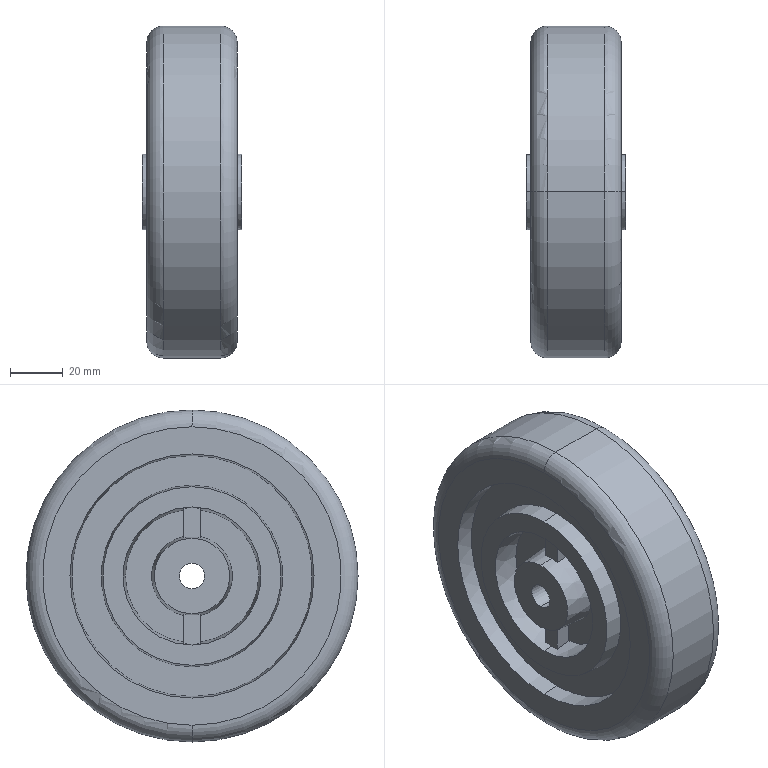Part | SolidWorks | features Cut 2, Draft 2, ICE 2, BossThin 1, Extrusion 1, Fillet 1, MirrorPattern 1 | 1 solid | 41 faces | box 37.592 x 125.73 x 125.73 mm | volume 351247 mm3 | plane 17 | cone 16 | cylinder 4 | torus 4 | commonest cylinder face diameters 9.652 x2 125.73 x2
STEP:
#1=CARTESIAN_POINT('',(18.796,-76.2,-39.751));
#2=VERTEX_POINT('',#1);
#3=CARTESIAN_POINT('',(18.796,-76.2,-30.099));
#4=VERTEX_POINT('',#3);
#5=CARTESIAN_POINT('',(18.796,-76.2,-34.925));
#6=DIRECTION('',(-1.,0.,0.));
#7=DIRECTION('',(0.,0.,1.));
#8=AXIS2_PLACEMENT_3D('',#5,#6,#7);
#9=CIRCLE('',#8,4.826);
#10=EDGE_CURVE('',#2,#4,#9,.T.);
#11=ORIENTED_EDGE('',*,*,#10,.F.);
#12=CARTESIAN_POINT('',(-18.796,-76.2,-39.751));
#13=VERTEX_POINT('',#12);
#14=CARTESIAN_POINT('',(18.796,-76.2,-39.751));
#15=DIRECTION('',(-1.,0.,0.));
#16=VECTOR('',#15,1000.);
#17=LINE('',#14,#16);
#18=EDGE_CURVE('',#2,#13,#17,.T.);
#19=ORIENTED_EDGE('',*,*,#18,.T.);
#20=CARTESIAN_POINT('',(-18.796,-76.2,-30.099));
#21=VERTEX_POINT('',#20);
#22=CARTESIAN_POINT('',(-18.796,-76.2,-34.925));
#23=DIRECTION('',(-1.,0.,0.));
#24=DIRECTION('',(0.,0.,1.));
#25=AXIS2_PLACEMENT_3D('',#22,#23,#24);
#26=CIRCLE('',#25,4.826);
#27=EDGE_CURVE('',#13,#21,#26,.T.);
#28=ORIENTED_EDGE('',*,*,#27,.T.);
#29=CARTESIAN_POINT('',(18.796,-76.2,-30.099));
#30=DIRECTION('',(-1.,0.,0.));
#31=VECTOR('',#30,1000.);
#32=LINE('',#29,#31);
#33=EDGE_CURVE('',#4,#21,#32,.T.);
#34=ORIENTED_EDGE('',*,*,#33,.F.);
#35=EDGE_LOOP('',(#11,#19,#28,#34));
#36=FACE_OUTER_BOUND('',#35,.T.);
#37=CARTESIAN_POINT('',(18.796,-76.2,-34.925));
#38=DIRECTION('',(-1.,0.,0.));
#39=DIRECTION('',(0.,0.,1.));
#40=AXIS2_PLACEMENT_3D('',#37,#38,#39);
#41=CYLINDRICAL_SURFACE('',#40,4.826);
#42=ADVANCED_FACE('',(#36),#41,.F.);
#43=CARTESIAN_POINT('',(10.795,-76.2,27.94));
#44=VERTEX_POINT('',#43);
#45=CARTESIAN_POINT('',(10.795,-76.2,-97.79));
#46=VERTEX_POINT('',#45);
#47=CARTESIAN_POINT('',(10.795,-76.2,-34.925));
#48=DIRECTION('',(-1.,0.,0.));
#49=DIRECTION('',(0.,0.,-1.));
#50=AXIS2_PLACEMENT_3D('',#47,#48,#49);
#51=CIRCLE('',#50,62.865);
#52=EDGE_CURVE('',#44,#46,#51,.T.);
#53=ORIENTED_EDGE('',*,*,#52,.F.);
#54=CARTESIAN_POINT('',(17.145,-76.2,21.59));
#55=VERTEX_POINT('',#54);
#56=CARTESIAN_POINT('',(10.795,-76.2,21.59));
#57=DIRECTION('',(0.,1.,0.));
#58=DIRECTION('',(0.,0.,1.));
#59=AXIS2_PLACEMENT_3D('',#56,#57,#58);
#60=CIRCLE('',#59,6.35);
#61=EDGE_CURVE('',#44,#55,#60,.T.);
#62=ORIENTED_EDGE('',*,*,#61,.T.);
#63=CARTESIAN_POINT('',(17.145,-76.2,-91.44));
#64=VERTEX_POINT('',#63);
#65=CARTESIAN_POINT('',(17.145,-76.2,-34.925));
#66=DIRECTION('',(1.,0.,0.));
#67=DIRECTION('',(0.,0.,-1.));
#68=AXIS2_PLACEMENT_3D('',#65,#66,#67);
#69=CIRCLE('',#68,56.515);
#70=EDGE_CURVE('',#64,#55,#69,.T.);
#71=ORIENTED_EDGE('',*,*,#70,.F.);
#72=CARTESIAN_POINT('',(10.795,-76.2,-91.44));
#73=DIRECTION('',(0.,-1.,0.));
#74=DIRECTION('',(0.,0.,-1.));
#75=AXIS2_PLACEMENT_3D('',#72,#73,#74);
#76=CIRCLE('',#75,6.35);
#77=EDGE_CURVE('',#46,#64,#76,.T.);
#78=ORIENTED_EDGE('',*,*,#77,.F.);
#79=EDGE_LOOP('',(#53,#62,#71,#78));
#80=FACE_OUTER_BOUND('',#79,.T.);
#81=CARTESIAN_POINT('',(10.795,-76.2,-34.925));
#82=DIRECTION('',(1.,0.,0.));
#83=DIRECTION('',(0.,0.,-1.));
#84=AXIS2_PLACEMENT_3D('',#81,#82,#83);
#85=TOROIDAL_SURFACE('',#84,56.515,6.35);
#86=ADVANCED_FACE('',(#80),#85,.T.);
#87=CARTESIAN_POINT('',(-17.145,-76.2,21.59));
#88=VERTEX_POINT('',#87);
#89=CARTESIAN_POINT('',(-17.145,-76.2,-91.44));
#90=VERTEX_POINT('',#89);
#91=CARTESIAN_POINT('',(-17.145,-76.2,-34.925));
#92=DIRECTION('',(-1.,0.,0.));
#93=DIRECTION('',(0.,0.,-1.));
#94=AXIS2_PLACEMENT_3D('',#91,#92,#93);
#95=CIRCLE('',#94,56.515);
#96=EDGE_CURVE('',#88,#90,#95,.T.);
#97=ORIENTED_EDGE('',*,*,#96,.F.);
#98=CARTESIAN_POINT('',(-10.795,-76.2,27.94));
#99=VERTEX_POINT('',#98);
#100=CARTESIAN_POINT('',(-10.795,-76.2,21.59));
#101=DIRECTION('',(0.,1.,0.));
#102=DIRECTION('',(0.,0.,1.));
#103=AXIS2_PLACEMENT_3D('',#100,#101,#102);
#104=CIRCLE('',#103,6.35);
#105=EDGE_CURVE('',#88,#99,#104,.T.);
#106=ORIENTED_EDGE('',*,*,#105,.T.);
#107=CARTESIAN_POINT('',(-10.795,-76.2,-97.79));
#108=VERTEX_POINT('',#107);
#109=CARTESIAN_POINT('',(-10.795,-76.2,-34.925));
#110=DIRECTION('',(1.,0.,0.));
#111=DIRECTION('',(0.,0.,-1.));
#112=AXIS2_PLACEMENT_3D('',#109,#110,#111);
#113=CIRCLE('',#112,62.865);
#114=EDGE_CURVE('',#108,#99,#113,.T.);
#115=ORIENTED_EDGE('',*,*,#114,.F.);
#116=CARTESIAN_POINT('',(-10.795,-76.2,-91.44));
#117=DIRECTION('',(0.,-1.,0.));
#118=DIRECTION('',(0.,0.,-1.));
#119=AXIS2_PLACEMENT_3D('',#116,#117,#118);
#120=CIRCLE('',#119,6.35);
#121=EDGE_CURVE('',#90,#108,#120,.T.);
#122=ORIENTED_EDGE('',*,*,#121,.F.);
#123=EDGE_LOOP('',(#97,#106,#115,#122));
#124=FACE_OUTER_BOUND('',#123,.T.);
#125=CARTESIAN_POINT('',(-10.795,-76.2,-34.925));
#126=DIRECTION('',(1.,0.,0.));
#127=DIRECTION('',(0.,0.,-1.));
#128=AXIS2_PLACEMENT_3D('',#125,#126,#127);
#129=TOROIDAL_SURFACE('',#128,56.515,6.35);
#130=ADVANCED_FACE('',(#124),#129,.T.);
#131=CARTESIAN_POINT('',(18.796,-76.2,-20.637));
#132=VERTEX_POINT('',#131);
#133=CARTESIAN_POINT('',(18.796,-76.2,-49.213));
#134=VERTEX_POINT('',#133);
#135=CARTESIAN_POINT('',(18.796,-76.2,-34.925));
#136=DIRECTION('',(1.,0.,0.));
#137=DIRECTION('',(0.,0.,-1.));
#138=AXIS2_PLACEMENT_3D('',#135,#136,#137);
#139=CIRCLE('',#138,14.288);
#140=EDGE_CURVE('',#132,#134,#139,.T.);
#141=ORIENTED_EDGE('',*,*,#140,.F.);
#142=CARTESIAN_POINT('',(6.985,-76.2,-19.604));
#143=VERTEX_POINT('',#142);
#144=CARTESIAN_POINT('',(18.796,-76.2,-20.638));
#145=DIRECTION('',(-0.9962,0.,0.08716));
#146=VECTOR('',#145,1000.);
#147=LINE('',#144,#146);
#148=EDGE_CURVE('',#132,#143,#147,.T.);
#149=ORIENTED_EDGE('',*,*,#148,.T.);
#150=CARTESIAN_POINT('',(6.985,-76.2,-50.246));
#151=VERTEX_POINT('',#150);
#152=CARTESIAN_POINT('',(6.985,-76.2,-34.925));
#153=DIRECTION('',(1.,0.,0.));
#154=DIRECTION('',(0.,0.,-1.));
#155=AXIS2_PLACEMENT_3D('',#152,#153,#154);
#156=CIRCLE('',#155,15.321);
#157=EDGE_CURVE('',#143,#151,#156,.T.);
#158=ORIENTED_EDGE('',*,*,#157,.T.);
#159=CARTESIAN_POINT('',(18.796,-76.2,-49.213));
#160=DIRECTION('',(-0.9962,0.,-0.08716));
#161=VECTOR('',#160,1000.);
#162=LINE('',#159,#161);
#163=EDGE_CURVE('',#134,#151,#162,.T.);
#164=ORIENTED_EDGE('',*,*,#163,.F.);
#165=EDGE_LOOP('',(#141,#149,#158,#164));
#166=FACE_OUTER_BOUND('',#165,.T.);
#167=CARTESIAN_POINT('',(18.796,-76.2,-34.925));
#168=DIRECTION('',(-1.,0.,0.));
#169=DIRECTION('',(0.,0.,-1.));
#170=AXIS2_PLACEMENT_3D('',#167,#168,#169);
#171=CONICAL_SURFACE('',#170,14.288,0.08727);
#172=ADVANCED_FACE('',(#166),#171,.T.);
#173=CARTESIAN_POINT('',(6.985,-76.2,-60.181));
#174=VERTEX_POINT('',#173);
#175=CARTESIAN_POINT('',(6.985,-76.2,-9.669));
#176=VERTEX_POINT('',#175);
#177=CARTESIAN_POINT('',(6.985,-76.2,-34.925));
#178=DIRECTION('',(-1.,0.,0.));
#179=DIRECTION('',(0.,0.,-1.));
#180=AXIS2_PLACEMENT_3D('',#177,#178,#179);
#181=CIRCLE('',#180,25.256);
#182=EDGE_CURVE('',#174,#176,#181,.T.);
#183=ORIENTED_EDGE('',*,*,#182,.T.);
#184=CARTESIAN_POINT('',(17.145,-76.2,-8.78));
#185=VERTEX_POINT('',#184);
#186=CARTESIAN_POINT('',(18.796,-76.2,-8.636));
#187=DIRECTION('',(0.9962,0.,0.08716));
#188=VECTOR('',#187,1000.);
#189=LINE('',#186,#188);
#190=EDGE_CURVE('',#176,#185,#189,.T.);
#191=ORIENTED_EDGE('',*,*,#190,.T.);
#192=CARTESIAN_POINT('',(17.145,-76.2,-61.07));
#193=VERTEX_POINT('',#192);
#194=CARTESIAN_POINT('',(17.145,-76.2,-34.925));
#195=DIRECTION('',(-1.,0.,0.));
#196=DIRECTION('',(0.,0.,-1.));
#197=AXIS2_PLACEMENT_3D('',#194,#195,#196);
#198=CIRCLE('',#197,26.145);
#199=EDGE_CURVE('',#193,#185,#198,.T.);
#200=ORIENTED_EDGE('',*,*,#199,.F.);
#201=CARTESIAN_POINT('',(18.796,-76.2,-61.214));
#202=DIRECTION('',(0.9962,0.,-0.08716));
#203=VECTOR('',#202,1000.);
#204=LINE('',#201,#203);
#205=EDGE_CURVE('',#174,#193,#204,.T.);
#206=ORIENTED_EDGE('',*,*,#205,.F.);
#207=EDGE_LOOP('',(#183,#191,#200,#206));
#208=FACE_OUTER_BOUND('',#207,.T.);
#209=CARTESIAN_POINT('',(18.796,-76.2,-34.925));
#210=DIRECTION('',(1.,0.,0.));
#211=DIRECTION('',(0.,0.,-1.));
#212=AXIS2_PLACEMENT_3D('',#209,#210,#211);
#213=CONICAL_SURFACE('',#212,26.289,0.08727);
#214=ADVANCED_FACE('',(#208),#213,.F.);
#215=CARTESIAN_POINT('',(17.145,-76.2,-68.724));
#216=VERTEX_POINT('',#215);
#217=CARTESIAN_POINT('',(17.145,-76.2,-1.126));
#218=VERTEX_POINT('',#217);
#219=CARTESIAN_POINT('',(17.145,-76.2,-34.925));
#220=DIRECTION('',(-1.,0.,0.));
#221=DIRECTION('',(0.,0.,-1.));
#222=AXIS2_PLACEMENT_3D('',#219,#220,#221);
#223=CIRCLE('',#222,33.799);
#224=EDGE_CURVE('',#216,#218,#223,.T.);
#225=ORIENTED_EDGE('',*,*,#224,.T.);
#226=CARTESIAN_POINT('',(10.414,-76.2,-0.5367));
#227=VERTEX_POINT('',#226);
#228=CARTESIAN_POINT('',(18.796,-76.2,-1.27));
#229=DIRECTION('',(-0.9962,0.,0.08716));
#230=VECTOR('',#229,1000.);
#231=LINE('',#228,#230);
#232=EDGE_CURVE('',#218,#227,#231,.T.);
#233=ORIENTED_EDGE('',*,*,#232,.T.);
#234=CARTESIAN_POINT('',(10.414,-76.2,-69.313));
#235=VERTEX_POINT('',#234);
#236=CARTESIAN_POINT('',(10.414,-76.2,-34.925));
#237=DIRECTION('',(-1.,0.,0.));
#238=DIRECTION('',(0.,0.,-1.));
#239=AXIS2_PLACEMENT_3D('',#236,#237,#238);
#240=CIRCLE('',#239,34.388);
#241=EDGE_CURVE('',#235,#227,#240,.T.);
#242=ORIENTED_EDGE('',*,*,#241,.F.);
#243=CARTESIAN_POINT('',(18.796,-76.2,-68.58));
#244=DIRECTION('',(-0.9962,0.,-0.08716));
#245=VECTOR('',#244,1000.);
#246=LINE('',#243,#245);
#247=EDGE_CURVE('',#216,#235,#246,.T.);
#248=ORIENTED_EDGE('',*,*,#247,.F.);
#249=EDGE_LOOP('',(#225,#233,#242,#248));
#250=FACE_OUTER_BOUND('',#249,.T.);
#251=CARTESIAN_POINT('',(18.796,-76.2,-34.925));
#252=DIRECTION('',(-1.,0.,0.));
#253=DIRECTION('',(0.,0.,-1.));
#254=AXIS2_PLACEMENT_3D('',#251,#252,#253);
#255=CONICAL_SURFACE('',#254,33.655,0.08727);
#256=ADVANCED_FACE('',(#250),#255,.T.);
#257=CARTESIAN_POINT('',(10.414,-76.2,-80.547));
#258=VERTEX_POINT('',#257);
#259=CARTESIAN_POINT('',(10.414,-76.2,10.697));
#260=VERTEX_POINT('',#259);
#261=CARTESIAN_POINT('',(10.414,-76.2,-34.925));
#262=DIRECTION('',(-1.,0.,0.));
#263=DIRECTION('',(0.,0.,-1.));
#264=AXIS2_PLACEMENT_3D('',#261,#262,#263);
#265=CIRCLE('',#264,45.622);
#266=EDGE_CURVE('',#258,#260,#265,.T.);
#267=ORIENTED_EDGE('',*,*,#266,.T.);
#268=CARTESIAN_POINT('',(17.145,-76.2,11.286));
#269=VERTEX_POINT('',#268);
#270=CARTESIAN_POINT('',(18.796,-76.2,11.43));
#271=DIRECTION('',(0.9962,0.,0.08716));
#272=VECTOR('',#271,1000.);
#273=LINE('',#270,#272);
#274=EDGE_CURVE('',#260,#269,#273,.T.);
#275=ORIENTED_EDGE('',*,*,#274,.T.);
#276=CARTESIAN_POINT('',(17.145,-76.2,-81.136));
#277=VERTEX_POINT('',#276);
#278=CARTESIAN_POINT('',(17.145,-76.2,-34.925));
#279=DIRECTION('',(-1.,0.,0.));
#280=DIRECTION('',(0.,0.,-1.));
#281=AXIS2_PLACEMENT_3D('',#278,#279,#280);
#282=CIRCLE('',#281,46.211);
#283=EDGE_CURVE('',#277,#269,#282,.T.);
#284=ORIENTED_EDGE('',*,*,#283,.F.);
#285=CARTESIAN_POINT('',(18.796,-76.2,-81.28));
#286=DIRECTION('',(0.9962,0.,-0.08716));
#287=VECTOR('',#286,1000.);
#288=LINE('',#285,#287);
#289=EDGE_CURVE('',#258,#277,#288,.T.);
#290=ORIENTED_EDGE('',*,*,#289,.F.);
#291=EDGE_LOOP('',(#267,#275,#284,#290));
#292=FACE_OUTER_BOUND('',#291,.T.);
#293=CARTESIAN_POINT('',(18.796,-76.2,-34.925));
#294=DIRECTION('',(1.,0.,0.));
#295=DIRECTION('',(0.,0.,-1.));
#296=AXIS2_PLACEMENT_3D('',#293,#294,#295);
#297=CONICAL_SURFACE('',#296,46.355,0.08727);
#298=ADVANCED_FACE('',(#292),#297,.F.);
#299=CARTESIAN_POINT('',(-17.145,-76.2,-68.724));
#300=VERTEX_POINT('',#299);
#301=CARTESIAN_POINT('',(-17.145,-76.2,-1.126));
#302=VERTEX_POINT('',#301);
#303=CARTESIAN_POINT('',(-17.145,-76.2,-34.925));
#304=DIRECTION('',(-1.,0.,0.));
#305=DIRECTION('',(0.,0.,-1.));
#306=AXIS2_PLACEMENT_3D('',#303,#304,#305);
#307=CIRCLE('',#306,33.799);
#308=EDGE_CURVE('',#300,#302,#307,.T.);
#309=ORIENTED_EDGE('',*,*,#308,.F.);
#310=CARTESIAN_POINT('',(-10.414,-76.2,-69.313));
#311=VERTEX_POINT('',#310);
#312=CARTESIAN_POINT('',(-18.796,-76.2,-68.58));
#313=DIRECTION('',(0.9962,0.,-0.08716));
#314=VECTOR('',#313,1000.);
#315=LINE('',#312,#314);
#316=EDGE_CURVE('',#300,#311,#315,.T.);
#317=ORIENTED_EDGE('',*,*,#316,.T.);
#318=CARTESIAN_POINT('',(-10.414,-76.2,-0.5367));
#319=VERTEX_POINT('',#318);
#320=CARTESIAN_POINT('',(-10.414,-76.2,-34.925));
#321=DIRECTION('',(-1.,0.,0.));
#322=DIRECTION('',(0.,0.,1.));
#323=AXIS2_PLACEMENT_3D('',#320,#321,#322);
#324=CIRCLE('',#323,34.388);
#325=EDGE_CURVE('',#311,#319,#324,.T.);
#326=ORIENTED_EDGE('',*,*,#325,.T.);
#327=CARTESIAN_POINT('',(-18.796,-76.2,-1.27));
#328=DIRECTION('',(0.9962,0.,0.08716));
#329=VECTOR('',#328,1000.);
#330=LINE('',#327,#329);
#331=EDGE_CURVE('',#302,#319,#330,.T.);
#332=ORIENTED_EDGE('',*,*,#331,.F.);
#333=EDGE_LOOP('',(#309,#317,#326,#332));
#334=FACE_OUTER_BOUND('',#333,.T.);
#335=CARTESIAN_POINT('',(-18.796,-76.2,-34.925));
#336=DIRECTION('',(1.,0.,0.));
#337=DIRECTION('',(0.,0.,1.));
#338=AXIS2_PLACEMENT_3D('',#335,#336,#337);
#339=CONICAL_SURFACE('',#338,33.655,0.08727);
#340=ADVANCED_FACE('',(#334),#339,.T.);
#341=CARTESIAN_POINT('',(-10.414,-76.2,-80.547));
#342=VERTEX_POINT('',#341);
#343=CARTESIAN_POINT('',(-10.414,-76.2,10.697));
#344=VERTEX_POINT('',#343);
#345=CARTESIAN_POINT('',(-10.414,-76.2,-34.925));
#346=DIRECTION('',(-1.,0.,0.));
#347=DIRECTION('',(0.,0.,1.));
#348=AXIS2_PLACEMENT_3D('',#345,#346,#347);
#349=CIRCLE('',#348,45.622);
#350=EDGE_CURVE('',#342,#344,#349,.T.);
#351=ORIENTED_EDGE('',*,*,#350,.F.);
#352=CARTESIAN_POINT('',(-17.145,-76.2,-81.136));
#353=VERTEX_POINT('',#352);
#354=CARTESIAN_POINT('',(-18.796,-76.2,-81.28));
#355=DIRECTION('',(-0.9962,0.,-0.08716));
#356=VECTOR('',#355,1000.);
#357=LINE('',#354,#356);
#358=EDGE_CURVE('',#342,#353,#357,.T.);
#359=ORIENTED_EDGE('',*,*,#358,.T.);
#360=CARTESIAN_POINT('',(-17.145,-76.2,11.286));
#361=VERTEX_POINT('',#360);
#362=CARTESIAN_POINT('',(-17.145,-76.2,-34.925));
#363=DIRECTION('',(-1.,0.,0.));
#364=DIRECTION('',(0.,0.,-1.));
#365=AXIS2_PLACEMENT_3D('',#362,#363,#364);
#366=CIRCLE('',#365,46.211);
#367=EDGE_CURVE('',#353,#361,#366,.T.);
#368=ORIENTED_EDGE('',*,*,#367,.T.);
#369=CARTESIAN_POINT('',(-18.796,-76.2,11.43));
#370=DIRECTION('',(-0.9962,0.,0.08716));
#371=VECTOR('',#370,1000.);
#372=LINE('',#369,#371);
#373=EDGE_CURVE('',#344,#361,#372,.T.);
#374=ORIENTED_EDGE('',*,*,#373,.F.);
#375=EDGE_LOOP('',(#351,#359,#368,#374));
#376=FACE_OUTER_BOUND('',#375,.T.);
#377=CARTESIAN_POINT('',(-18.796,-76.2,-34.925));
#378=DIRECTION('',(-1.,0.,0.));
#379=DIRECTION('',(0.,0.,1.));
#380=AXIS2_PLACEMENT_3D('',#377,#378,#379);
#381=CONICAL_SURFACE('',#380,46.355,0.08727);
#382=ADVANCED_FACE('',(#376),#381,.F.);
#383=ORIENTED_EDGE('',*,*,#114,.T.);
#384=CARTESIAN_POINT('',(-17.145,-76.2,27.94));
#385=DIRECTION('',(1.,0.,0.));
#386=VECTOR('',#385,1000.);
#387=LINE('',#384,#386);
#388=EDGE_CURVE('',#99,#44,#387,.T.);
#389=ORIENTED_EDGE('',*,*,#388,.T.);
#390=ORIENTED_EDGE('',*,*,#52,.T.);
#391=CARTESIAN_POINT('',(-17.145,-76.2,-97.79));
#392=DIRECTION('',(1.,0.,0.));
#393=VECTOR('',#392,1000.);
#394=LINE('',#391,#393);
#395=EDGE_CURVE('',#108,#46,#394,.T.);
#396=ORIENTED_EDGE('',*,*,#395,.F.);
#397=EDGE_LOOP('',(#383,#389,#390,#396));
#398=FACE_OUTER_BOUND('',#397,.T.);
#399=CARTESIAN_POINT('',(-17.145,-76.2,-34.925));
#400=DIRECTION('',(1.,0.,0.));
#401=DIRECTION('',(0.,0.,-1.));
#402=AXIS2_PLACEMENT_3D('',#399,#400,#401);
#403=CYLINDRICAL_SURFACE('',#402,62.865);
#404=ADVANCED_FACE('',(#398),#403,.T.);
#405=CARTESIAN_POINT('',(-18.796,-76.2,-20.637));
#406=VERTEX_POINT('',#405);
#407=CARTESIAN_POINT('',(-18.796,-76.2,-49.213));
#408=VERTEX_POINT('',#407);
#409=CARTESIAN_POINT('',(-18.796,-76.2,-34.925));
#410=DIRECTION('',(1.,0.,0.));
#411=DIRECTION('',(0.,0.,-1.));
#412=AXIS2_PLACEMENT_3D('',#409,#410,#411);
#413=CIRCLE('',#412,14.288);
#414=EDGE_CURVE('',#406,#408,#413,.T.);
#415=ORIENTED_EDGE('',*,*,#414,.T.);
#416=CARTESIAN_POINT('',(-13.335,-76.2,-49.69));
#417=VERTEX_POINT('',#416);
#418=CARTESIAN_POINT('',(-18.796,-76.2,-49.213));
#419=DIRECTION('',(0.9962,0.,-0.08716));
#420=VECTOR('',#419,1000.);
#421=LINE('',#418,#420);
#422=EDGE_CURVE('',#408,#417,#421,.T.);
#423=ORIENTED_EDGE('',*,*,#422,.T.);
#424=CARTESIAN_POINT('',(-13.335,-79.375,-49.345));
#425=VERTEX_POINT('',#424);
#426=CARTESIAN_POINT('',(-13.335,-76.2,-34.925));
#427=DIRECTION('',(-1.,0.,0.));
#428=DIRECTION('',(0.,0.,-1.));
#429=AXIS2_PLACEMENT_3D('',#426,#427,#428);
#430=CIRCLE('',#429,14.765);
#431=EDGE_CURVE('',#417,#425,#430,.T.);
#432=ORIENTED_EDGE('',*,*,#431,.T.);
#433=CARTESIAN_POINT('',(-6.985,-79.375,-49.913));
#434=VERTEX_POINT('',#433);
#435=CARTESIAN_POINT('',(-13.335,-79.375,-49.345));
#436=CARTESIAN_POINT('',(-13.061,-79.375,-49.369));
#437=CARTESIAN_POINT('',(-12.787,-79.375,-49.394));
#438=CARTESIAN_POINT('',(-12.513,-79.375,-49.418));
#439=CARTESIAN_POINT('',(-10.671,-79.375,-49.584));
#440=CARTESIAN_POINT('',(-8.828,-79.375,-49.748));
#441=CARTESIAN_POINT('',(-6.985,-79.375,-49.913));
#442=B_SPLINE_CURVE_WITH_KNOTS('',3,(#435,#436,#437,#438,#439,#440,#441),.UNSPECIFIED.,.F.,.F.,(4,3,4),(0.01102,0.01184,0.01739),.UNSPECIFIED.);
#443=EDGE_CURVE('',#425,#434,#442,.T.);
#444=ORIENTED_EDGE('',*,*,#443,.T.);
#445=CARTESIAN_POINT('',(-6.985,-79.375,-19.937));
#446=VERTEX_POINT('',#445);
#447=CARTESIAN_POINT('',(-6.985,-76.2,-34.925));
#448=DIRECTION('',(-1.,0.,0.));
#449=DIRECTION('',(0.,0.,1.));
#450=AXIS2_PLACEMENT_3D('',#447,#448,#449);
#451=CIRCLE('',#450,15.321);
#452=EDGE_CURVE('',#434,#446,#451,.T.);
#453=ORIENTED_EDGE('',*,*,#452,.T.);
#454=CARTESIAN_POINT('',(-13.335,-79.375,-20.505));
#455=VERTEX_POINT('',#454);
#456=CARTESIAN_POINT('',(-6.985,-79.375,-19.937));
#457=CARTESIAN_POINT('',(-8.828,-79.375,-20.102));
#458=CARTESIAN_POINT('',(-10.671,-79.375,-20.266));
#459=CARTESIAN_POINT('',(-12.513,-79.375,-20.432));
#460=CARTESIAN_POINT('',(-12.787,-79.375,-20.456));
#461=CARTESIAN_POINT('',(-13.061,-79.375,-20.481));
#462=CARTESIAN_POINT('',(-13.335,-79.375,-20.505));
#463=B_SPLINE_CURVE_WITH_KNOTS('',3,(#456,#457,#458,#459,#460,#461,#462),.UNSPECIFIED.,.F.,.F.,(4,3,4),(0.006292,0.01184,0.01267),.UNSPECIFIED.);
#464=EDGE_CURVE('',#446,#455,#463,.T.);
#465=ORIENTED_EDGE('',*,*,#464,.T.);
#466=CARTESIAN_POINT('',(-13.335,-76.2,-20.16));
#467=VERTEX_POINT('',#466);
#468=CARTESIAN_POINT('',(-13.335,-76.2,-34.925));
#469=DIRECTION('',(-1.,0.,0.));
#470=DIRECTION('',(0.,0.,-1.));
#471=AXIS2_PLACEMENT_3D('',#468,#469,#470);
#472=CIRCLE('',#471,14.765);
#473=EDGE_CURVE('',#455,#467,#472,.T.);
#474=ORIENTED_EDGE('',*,*,#473,.T.);
#475=CARTESIAN_POINT('',(-18.796,-76.2,-20.638));
#476=DIRECTION('',(0.9962,0.,0.08716));
#477=VECTOR('',#476,1000.);
#478=LINE('',#475,#477);
#479=EDGE_CURVE('',#406,#467,#478,.T.);
#480=ORIENTED_EDGE('',*,*,#479,.F.);
#481=EDGE_LOOP('',(#415,#423,#432,#444,#453,#465,#474,#480));
#482=FACE_OUTER_BOUND('',#481,.T.);
#483=CARTESIAN_POINT('',(-18.796,-76.2,-34.925));
#484=DIRECTION('',(1.,0.,0.));
#485=DIRECTION('',(0.,0.,1.));
#486=AXIS2_PLACEMENT_3D('',#483,#484,#485);
#487=CONICAL_SURFACE('',#486,14.288,0.08727);
#488=ADVANCED_FACE('',(#482),#487,.T.);
#489=CARTESIAN_POINT('',(-13.335,-76.2,-60.736));
#490=VERTEX_POINT('',#489);
#491=CARTESIAN_POINT('',(-13.335,-79.375,-60.54));
#492=VERTEX_POINT('',#491);
#493=CARTESIAN_POINT('',(-13.335,-76.2,-34.925));
#494=DIRECTION('',(-1.,0.,0.));
#495=DIRECTION('',(0.,0.,-1.));
#496=AXIS2_PLACEMENT_3D('',#493,#494,#495);
#497=CIRCLE('',#496,25.811);
#498=EDGE_CURVE('',#490,#492,#497,.T.);
#499=ORIENTED_EDGE('',*,*,#498,.F.);
#500=CARTESIAN_POINT('',(-17.145,-76.2,-61.07));
#501=VERTEX_POINT('',#500);
#502=CARTESIAN_POINT('',(-18.796,-76.2,-61.214));
#503=DIRECTION('',(-0.9962,0.,-0.08716));
#504=VECTOR('',#503,1000.);
#505=LINE('',#502,#504);
#506=EDGE_CURVE('',#490,#501,#505,.T.);
#507=ORIENTED_EDGE('',*,*,#506,.T.);
#508=CARTESIAN_POINT('',(-17.145,-76.2,-8.78));
#509=VERTEX_POINT('',#508);
#510=CARTESIAN_POINT('',(-17.145,-76.2,-34.925));
#511=DIRECTION('',(-1.,0.,0.));
#512=DIRECTION('',(0.,0.,-1.));
#513=AXIS2_PLACEMENT_3D('',#510,#511,#512);
#514=CIRCLE('',#513,26.145);
#515=EDGE_CURVE('',#501,#509,#514,.T.);
#516=ORIENTED_EDGE('',*,*,#515,.T.);
#517=CARTESIAN_POINT('',(-13.335,-76.2,-9.114));
#518=VERTEX_POINT('',#517);
#519=CARTESIAN_POINT('',(-18.796,-76.2,-8.636));
#520=DIRECTION('',(-0.9962,0.,0.08716));
#521=VECTOR('',#520,1000.);
#522=LINE('',#519,#521);
#523=EDGE_CURVE('',#518,#509,#522,.T.);
#524=ORIENTED_EDGE('',*,*,#523,.F.);
#525=CARTESIAN_POINT('',(-13.335,-79.375,-9.31));
#526=VERTEX_POINT('',#525);
#527=CARTESIAN_POINT('',(-13.335,-76.2,-34.925));
#528=DIRECTION('',(-1.,0.,0.));
#529=DIRECTION('',(0.,0.,-1.));
#530=AXIS2_PLACEMENT_3D('',#527,#528,#529);
#531=CIRCLE('',#530,25.811);
#532=EDGE_CURVE('',#526,#518,#531,.T.);
#533=ORIENTED_EDGE('',*,*,#532,.F.);
#534=CARTESIAN_POINT('',(-6.985,-79.375,-9.87));
#535=VERTEX_POINT('',#534);
#536=CARTESIAN_POINT('',(-6.985,-79.375,-9.87));
#537=CARTESIAN_POINT('',(-8.549,-79.375,-9.732));
#538=CARTESIAN_POINT('',(-10.113,-79.375,-9.594));
#539=CARTESIAN_POINT('',(-11.676,-79.375,-9.456));
#540=CARTESIAN_POINT('',(-12.229,-79.375,-9.407));
#541=CARTESIAN_POINT('',(-12.782,-79.375,-9.359));
#542=CARTESIAN_POINT('',(-13.335,-79.375,-9.31));
#543=B_SPLINE_CURVE_WITH_KNOTS('',3,(#536,#537,#538,#539,#540,#541,#542),.UNSPECIFIED.,.F.,.F.,(4,3,4),(0.02187,0.02658,0.02824),.UNSPECIFIED.);
#544=EDGE_CURVE('',#535,#526,#543,.T.);
#545=ORIENTED_EDGE('',*,*,#544,.F.);
#546=CARTESIAN_POINT('',(-6.985,-79.375,-59.98));
#547=VERTEX_POINT('',#546);
#548=CARTESIAN_POINT('',(-6.985,-76.2,-34.925));
#549=DIRECTION('',(-1.,0.,0.));
#550=DIRECTION('',(0.,0.,1.));
#551=AXIS2_PLACEMENT_3D('',#548,#549,#550);
#552=CIRCLE('',#551,25.256);
#553=EDGE_CURVE('',#547,#535,#552,.T.);
#554=ORIENTED_EDGE('',*,*,#553,.F.);
#555=CARTESIAN_POINT('',(-13.335,-79.375,-60.54));
#556=CARTESIAN_POINT('',(-12.782,-79.375,-60.491));
#557=CARTESIAN_POINT('',(-12.229,-79.375,-60.443));
#558=CARTESIAN_POINT('',(-11.676,-79.375,-60.394));
#559=CARTESIAN_POINT('',(-10.113,-79.375,-60.256));
#560=CARTESIAN_POINT('',(-8.549,-79.375,-60.118));
#561=CARTESIAN_POINT('',(-6.985,-79.375,-59.98));
#562=B_SPLINE_CURVE_WITH_KNOTS('',3,(#555,#556,#557,#558,#559,#560,#561),.UNSPECIFIED.,.F.,.F.,(4,3,4),(0.02491,0.02658,0.03129),.UNSPECIFIED.);
#563=EDGE_CURVE('',#492,#547,#562,.T.);
#564=ORIENTED_EDGE('',*,*,#563,.F.);
#565=EDGE_LOOP('',(#499,#507,#516,#524,#533,#545,#554,#564));
#566=FACE_OUTER_BOUND('',#565,.T.);
#567=CARTESIAN_POINT('',(-18.796,-76.2,-34.925));
#568=DIRECTION('',(-1.,0.,0.));
#569=DIRECTION('',(0.,0.,1.));
#570=AXIS2_PLACEMENT_3D('',#567,#568,#569);
#571=CONICAL_SURFACE('',#570,26.289,0.08727);
#572=ADVANCED_FACE('',(#566),#571,.F.);
#573=ORIENTED_EDGE('',*,*,#506,.F.);
#574=CARTESIAN_POINT('',(-13.335,-73.025,-60.54));
#575=VERTEX_POINT('',#574);
#576=CARTESIAN_POINT('',(-13.335,-76.2,-34.925));
#577=DIRECTION('',(-1.,0.,0.));
#578=DIRECTION('',(0.,0.,-1.));
#579=AXIS2_PLACEMENT_3D('',#576,#577,#578);
#580=CIRCLE('',#579,25.811);
#581=EDGE_CURVE('',#575,#490,#580,.T.);
#582=ORIENTED_EDGE('',*,*,#581,.F.);
#583=CARTESIAN_POINT('',(-6.985,-73.025,-59.98));
#584=VERTEX_POINT('',#583);
#585=CARTESIAN_POINT('',(-13.335,-73.025,-60.54));
#586=CARTESIAN_POINT('',(-12.782,-73.025,-60.491));
#587=CARTESIAN_POINT('',(-12.229,-73.025,-60.443));
#588=CARTESIAN_POINT('',(-11.676,-73.025,-60.394));
#589=CARTESIAN_POINT('',(-10.113,-73.025,-60.256));
#590=CARTESIAN_POINT('',(-8.549,-73.025,-60.118));
#591=CARTESIAN_POINT('',(-6.985,-73.025,-59.98));
#592=B_SPLINE_CURVE_WITH_KNOTS('',3,(#585,#586,#587,#588,#589,#590,#591),.UNSPECIFIED.,.F.,.F.,(4,3,4),(0.02491,0.02658,0.03129),.UNSPECIFIED.);
#593=EDGE_CURVE('',#575,#584,#592,.T.);
#594=ORIENTED_EDGE('',*,*,#593,.T.);
#595=CARTESIAN_POINT('',(-6.985,-73.025,-9.87));
#596=VERTEX_POINT('',#595);
#597=CARTESIAN_POINT('',(-6.985,-76.2,-34.925));
#598=DIRECTION('',(-1.,0.,0.));
#599=DIRECTION('',(0.,0.,1.));
#600=AXIS2_PLACEMENT_3D('',#597,#598,#599);
#601=CIRCLE('',#600,25.256);
#602=EDGE_CURVE('',#596,#584,#601,.T.);
#603=ORIENTED_EDGE('',*,*,#602,.F.);
#604=CARTESIAN_POINT('',(-13.335,-73.025,-9.31));
#605=VERTEX_POINT('',#604);
#606=CARTESIAN_POINT('',(-6.985,-73.025,-9.87));
#607=CARTESIAN_POINT('',(-8.549,-73.025,-9.732));
#608=CARTESIAN_POINT('',(-10.113,-73.025,-9.594));
#609=CARTESIAN_POINT('',(-11.676,-73.025,-9.456));
#610=CARTESIAN_POINT('',(-12.229,-73.025,-9.407));
#611=CARTESIAN_POINT('',(-12.782,-73.025,-9.359));
#612=CARTESIAN_POINT('',(-13.335,-73.025,-9.31));
#613=B_SPLINE_CURVE_WITH_KNOTS('',3,(#606,#607,#608,#609,#610,#611,#612),.UNSPECIFIED.,.F.,.F.,(4,3,4),(0.02187,0.02658,0.02824),.UNSPECIFIED.);
#614=EDGE_CURVE('',#596,#605,#613,.T.);
#615=ORIENTED_EDGE('',*,*,#614,.T.);
#616=CARTESIAN_POINT('',(-13.335,-76.2,-34.925));
#617=DIRECTION('',(-1.,0.,0.));
#618=DIRECTION('',(0.,0.,-1.));
#619=AXIS2_PLACEMENT_3D('',#616,#617,#618);
#620=CIRCLE('',#619,25.811);
#621=EDGE_CURVE('',#518,#605,#620,.T.);
#622=ORIENTED_EDGE('',*,*,#621,.F.);
#623=ORIENTED_EDGE('',*,*,#523,.T.);
#624=CARTESIAN_POINT('',(-17.145,-76.2,-34.925));
#625=DIRECTION('',(-1.,0.,0.));
#626=DIRECTION('',(0.,0.,-1.));
#627=AXIS2_PLACEMENT_3D('',#624,#625,#626);
#628=CIRCLE('',#627,26.145);
#629=EDGE_CURVE('',#509,#501,#628,.T.);
#630=ORIENTED_EDGE('',*,*,#629,.T.);
#631=EDGE_LOOP('',(#573,#582,#594,#603,#615,#622,#623,#630));
#632=FACE_OUTER_BOUND('',#631,.T.);
#633=CARTESIAN_POINT('',(-18.796,-76.2,-34.925));
#634=DIRECTION('',(-1.,0.,0.));
#635=DIRECTION('',(0.,0.,1.));
#636=AXIS2_PLACEMENT_3D('',#633,#634,#635);
#637=CONICAL_SURFACE('',#636,26.289,0.08727);
#638=ADVANCED_FACE('',(#632),#637,.F.);
#639=ORIENTED_EDGE('',*,*,#553,.T.);
#640=CARTESIAN_POINT('',(-6.985,-79.375,-20.638));
#641=DIRECTION('',(0.,0.,1.));
#642=VECTOR('',#641,1000.);
#643=LINE('',#640,#642);
#644=EDGE_CURVE('',#446,#535,#643,.T.);
#645=ORIENTED_EDGE('',*,*,#644,.F.);
#646=ORIENTED_EDGE('',*,*,#452,.F.);
#647=CARTESIAN_POINT('',(-6.985,-79.375,-61.07));
#648=DIRECTION('',(0.,0.,1.));
#649=VECTOR('',#648,1000.);
#650=LINE('',#647,#649);
#651=EDGE_CURVE('',#547,#434,#650,.T.);
#652=ORIENTED_EDGE('',*,*,#651,.F.);
#653=EDGE_LOOP('',(#639,#645,#646,#652));
#654=FACE_OUTER_BOUND('',#653,.T.);
#655=CARTESIAN_POINT('',(-6.985,-76.2,-34.925));
#656=DIRECTION('',(-1.,0.,0.));
#657=DIRECTION('',(0.,0.,1.));
#658=AXIS2_PLACEMENT_3D('',#655,#656,#657);
#659=PLANE('',#658);
#660=ADVANCED_FACE('',(#654),#659,.T.);
#661=ORIENTED_EDGE('',*,*,#422,.F.);
#662=CARTESIAN_POINT('',(-18.796,-76.2,-34.925));
#663=DIRECTION('',(1.,0.,0.));
#664=DIRECTION('',(0.,0.,-1.));
#665=AXIS2_PLACEMENT_3D('',#662,#663,#664);
#666=CIRCLE('',#665,14.288);
#667=EDGE_CURVE('',#408,#406,#666,.T.);
#668=ORIENTED_EDGE('',*,*,#667,.T.);
#669=ORIENTED_EDGE('',*,*,#479,.T.);
#670=CARTESIAN_POINT('',(-13.335,-73.025,-20.505));
#671=VERTEX_POINT('',#670);
#672=CARTESIAN_POINT('',(-13.335,-76.2,-34.925));
#673=DIRECTION('',(-1.,0.,0.));
#674=DIRECTION('',(0.,0.,-1.));
#675=AXIS2_PLACEMENT_3D('',#672,#673,#674);
#676=CIRCLE('',#675,14.765);
#677=EDGE_CURVE('',#467,#671,#676,.T.);
#678=ORIENTED_EDGE('',*,*,#677,.T.);
#679=CARTESIAN_POINT('',(-6.985,-73.025,-19.937));
#680=VERTEX_POINT('',#679);
#681=CARTESIAN_POINT('',(-6.985,-73.025,-19.937));
#682=CARTESIAN_POINT('',(-8.828,-73.025,-20.102));
#683=CARTESIAN_POINT('',(-10.671,-73.025,-20.266));
#684=CARTESIAN_POINT('',(-12.513,-73.025,-20.432));
#685=CARTESIAN_POINT('',(-12.787,-73.025,-20.456));
#686=CARTESIAN_POINT('',(-13.061,-73.025,-20.481));
#687=CARTESIAN_POINT('',(-13.335,-73.025,-20.505));
#688=B_SPLINE_CURVE_WITH_KNOTS('',3,(#681,#682,#683,#684,#685,#686,#687),.UNSPECIFIED.,.F.,.F.,(4,3,4),(0.006292,0.01184,0.01267),.UNSPECIFIED.);
#689=EDGE_CURVE('',#680,#671,#688,.T.);
#690=ORIENTED_EDGE('',*,*,#689,.F.);
#691=CARTESIAN_POINT('',(-6.985,-73.025,-49.913));
#692=VERTEX_POINT('',#691);
#693=CARTESIAN_POINT('',(-6.985,-76.2,-34.925));
#694=DIRECTION('',(-1.,0.,0.));
#695=DIRECTION('',(0.,0.,1.));
#696=AXIS2_PLACEMENT_3D('',#693,#694,#695);
#697=CIRCLE('',#696,15.321);
#698=EDGE_CURVE('',#680,#692,#697,.T.);
#699=ORIENTED_EDGE('',*,*,#698,.T.);
#700=CARTESIAN_POINT('',(-13.335,-73.025,-49.345));
#701=VERTEX_POINT('',#700);
#702=CARTESIAN_POINT('',(-13.335,-73.025,-49.345));
#703=CARTESIAN_POINT('',(-13.061,-73.025,-49.369));
#704=CARTESIAN_POINT('',(-12.787,-73.025,-49.394));
#705=CARTESIAN_POINT('',(-12.513,-73.025,-49.418));
#706=CARTESIAN_POINT('',(-10.671,-73.025,-49.584));
#707=CARTESIAN_POINT('',(-8.828,-73.025,-49.748));
#708=CARTESIAN_POINT('',(-6.985,-73.025,-49.913));
#709=B_SPLINE_CURVE_WITH_KNOTS('',3,(#702,#703,#704,#705,#706,#707,#708),.UNSPECIFIED.,.F.,.F.,(4,3,4),(0.01102,0.01184,0.01739),.UNSPECIFIED.);
#710=EDGE_CURVE('',#701,#692,#709,.T.);
#711=ORIENTED_EDGE('',*,*,#710,.F.);
#712=CARTESIAN_POINT('',(-13.335,-76.2,-34.925));
#713=DIRECTION('',(-1.,0.,0.));
#714=DIRECTION('',(0.,0.,-1.));
#715=AXIS2_PLACEMENT_3D('',#712,#713,#714);
#716=CIRCLE('',#715,14.765);
#717=EDGE_CURVE('',#701,#417,#716,.T.);
#718=ORIENTED_EDGE('',*,*,#717,.T.);
#719=EDGE_LOOP('',(#661,#668,#669,#678,#690,#699,#711,#718));
#720=FACE_OUTER_BOUND('',#719,.T.);
#721=CARTESIAN_POINT('',(-18.796,-76.2,-34.925));
#722=DIRECTION('',(1.,0.,0.));
#723=DIRECTION('',(0.,0.,1.));
#724=AXIS2_PLACEMENT_3D('',#721,#722,#723);
#725=CONICAL_SURFACE('',#724,14.288,0.08727);
#726=ADVANCED_FACE('',(#720),#725,.T.);
#727=CARTESIAN_POINT('',(-6.985,-73.025,-20.638));
#728=DIRECTION('',(0.,0.,1.));
#729=VECTOR('',#728,1000.);
#730=LINE('',#727,#729);
#731=EDGE_CURVE('',#680,#596,#730,.T.);
#732=ORIENTED_EDGE('',*,*,#731,.T.);
#733=ORIENTED_EDGE('',*,*,#602,.T.);
#734=CARTESIAN_POINT('',(-6.985,-73.025,-61.07));
#735=DIRECTION('',(0.,0.,1.));
#736=VECTOR('',#735,1000.);
#737=LINE('',#734,#736);
#738=EDGE_CURVE('',#584,#692,#737,.T.);
#739=ORIENTED_EDGE('',*,*,#738,.T.);
#740=ORIENTED_EDGE('',*,*,#698,.F.);
#741=EDGE_LOOP('',(#732,#733,#739,#740));
#742=FACE_OUTER_BOUND('',#741,.T.);
#743=CARTESIAN_POINT('',(-6.985,-76.2,-34.925));
#744=DIRECTION('',(-1.,0.,0.));
#745=DIRECTION('',(0.,0.,1.));
#746=AXIS2_PLACEMENT_3D('',#743,#744,#745);
#747=PLANE('',#746);
#748=ADVANCED_FACE('',(#742),#747,.T.);
#749=ORIENTED_EDGE('',*,*,#388,.F.);
#750=CARTESIAN_POINT('',(-10.795,-76.2,-34.925));
#751=DIRECTION('',(1.,0.,0.));
#752=DIRECTION('',(0.,0.,-1.));
#753=AXIS2_PLACEMENT_3D('',#750,#751,#752);
#754=CIRCLE('',#753,62.865);
#755=EDGE_CURVE('',#99,#108,#754,.T.);
#756=ORIENTED_EDGE('',*,*,#755,.T.);
#757=ORIENTED_EDGE('',*,*,#395,.T.);
#758=CARTESIAN_POINT('',(10.795,-76.2,-34.925));
#759=DIRECTION('',(-1.,0.,0.));
#760=DIRECTION('',(0.,0.,-1.));
#761=AXIS2_PLACEMENT_3D('',#758,#759,#760);
#762=CIRCLE('',#761,62.865);
#763=EDGE_CURVE('',#46,#44,#762,.T.);
#764=ORIENTED_EDGE('',*,*,#763,.T.);
#765=EDGE_LOOP('',(#749,#756,#757,#764));
#766=FACE_OUTER_BOUND('',#765,.T.);
#767=CARTESIAN_POINT('',(-17.145,-76.2,-34.925));
#768=DIRECTION('',(1.,0.,0.));
#769=DIRECTION('',(0.,0.,-1.));
#770=AXIS2_PLACEMENT_3D('',#767,#768,#769);
#771=CYLINDRICAL_SURFACE('',#770,62.865);
#772=ADVANCED_FACE('',(#766),#771,.T.);
#773=CARTESIAN_POINT('',(-17.145,-76.2,-34.925));
#774=DIRECTION('',(-1.,0.,0.));
#775=DIRECTION('',(0.,0.,-1.));
#776=AXIS2_PLACEMENT_3D('',#773,#774,#775);
#777=CIRCLE('',#776,56.515);
#778=EDGE_CURVE('',#90,#88,#777,.T.);
#779=ORIENTED_EDGE('',*,*,#778,.T.);
#780=ORIENTED_EDGE('',*,*,#96,.T.);
#781=EDGE_LOOP('',(#779,#780));
#782=FACE_OUTER_BOUND('',#781,.T.);
#783=CARTESIAN_POINT('',(-17.145,-76.2,-34.925));
#784=DIRECTION('',(-1.,0.,0.));
#785=DIRECTION('',(0.,0.,-1.));
#786=AXIS2_PLACEMENT_3D('',#783,#784,#785);
#787=CIRCLE('',#786,46.211);
#788=EDGE_CURVE('',#361,#353,#787,.T.);
#789=ORIENTED_EDGE('',*,*,#788,.F.);
#790=ORIENTED_EDGE('',*,*,#367,.F.);
#791=EDGE_LOOP('',(#789,#790));
#792=FACE_BOUND('',#791,.T.);
#793=CARTESIAN_POINT('',(-17.145,-76.2,-34.925));
#794=DIRECTION('',(1.,0.,0.));
#795=DIRECTION('',(0.,0.,-1.));
#796=AXIS2_PLACEMENT_3D('',#793,#794,#795);
#797=PLANE('',#796);
#798=ADVANCED_FACE('',(#782,#792),#797,.F.);
#799=ORIENTED_EDGE('',*,*,#70,.T.);
#800=CARTESIAN_POINT('',(17.145,-76.2,-34.925));
#801=DIRECTION('',(1.,0.,0.));
#802=DIRECTION('',(0.,0.,-1.));
#803=AXIS2_PLACEMENT_3D('',#800,#801,#802);
#804=CIRCLE('',#803,56.515);
#805=EDGE_CURVE('',#55,#64,#804,.T.);
#806=ORIENTED_EDGE('',*,*,#805,.T.);
#807=EDGE_LOOP('',(#799,#806));
#808=FACE_OUTER_BOUND('',#807,.T.);
#809=ORIENTED_EDGE('',*,*,#283,.T.);
#810=CARTESIAN_POINT('',(17.145,-76.2,-34.925));
#811=DIRECTION('',(-1.,0.,0.));
#812=DIRECTION('',(0.,0.,-1.));
#813=AXIS2_PLACEMENT_3D('',#810,#811,#812);
#814=CIRCLE('',#813,46.211);
#815=EDGE_CURVE('',#269,#277,#814,.T.);
#816=ORIENTED_EDGE('',*,*,#815,.T.);
#817=EDGE_LOOP('',(#809,#816));
#818=FACE_BOUND('',#817,.T.);
#819=CARTESIAN_POINT('',(17.145,-76.2,-34.925));
#820=DIRECTION('',(1.,0.,0.));
#821=DIRECTION('',(0.,0.,-1.));
#822=AXIS2_PLACEMENT_3D('',#819,#820,#821);
#823=PLANE('',#822);
#824=ADVANCED_FACE('',(#808,#818),#823,.T.);
#825=ORIENTED_EDGE('',*,*,#358,.F.);
#826=CARTESIAN_POINT('',(-10.414,-76.2,-34.925));
#827=DIRECTION('',(-1.,0.,0.));
#828=DIRECTION('',(0.,0.,1.));
#829=AXIS2_PLACEMENT_3D('',#826,#827,#828);
#830=CIRCLE('',#829,45.622);
#831=EDGE_CURVE('',#344,#342,#830,.T.);
#832=ORIENTED_EDGE('',*,*,#831,.F.);
#833=ORIENTED_EDGE('',*,*,#373,.T.);
#834=ORIENTED_EDGE('',*,*,#788,.T.);
#835=EDGE_LOOP('',(#825,#832,#833,#834));
#836=FACE_OUTER_BOUND('',#835,.T.);
#837=CARTESIAN_POINT('',(-18.796,-76.2,-34.925));
#838=DIRECTION('',(-1.,0.,0.));
#839=DIRECTION('',(0.,0.,1.));
#840=AXIS2_PLACEMENT_3D('',#837,#838,#839);
#841=CONICAL_SURFACE('',#840,46.355,0.08727);
#842=ADVANCED_FACE('',(#836),#841,.F.);
#843=CARTESIAN_POINT('',(-10.414,-76.2,-34.925));
#844=DIRECTION('',(-1.,0.,0.));
#845=DIRECTION('',(0.,0.,1.));
#846=AXIS2_PLACEMENT_3D('',#843,#844,#845);
#847=CIRCLE('',#846,34.388);
#848=EDGE_CURVE('',#319,#311,#847,.T.);
#849=ORIENTED_EDGE('',*,*,#848,.F.);
#850=ORIENTED_EDGE('',*,*,#325,.F.);
#851=EDGE_LOOP('',(#849,#850));
#852=FACE_BOUND('',#851,.T.);
#853=ORIENTED_EDGE('',*,*,#831,.T.);
#854=ORIENTED_EDGE('',*,*,#350,.T.);
#855=EDGE_LOOP('',(#853,#854));
#856=FACE_OUTER_BOUND('',#855,.T.);
#857=CARTESIAN_POINT('',(-10.414,-76.2,-34.925));
#858=DIRECTION('',(-1.,0.,0.));
#859=DIRECTION('',(0.,0.,1.));
#860=AXIS2_PLACEMENT_3D('',#857,#858,#859);
#861=PLANE('',#860);
#862=ADVANCED_FACE('',(#852,#856),#861,.T.);
#863=ORIENTED_EDGE('',*,*,#316,.F.);
#864=CARTESIAN_POINT('',(-17.145,-76.2,-34.925));
#865=DIRECTION('',(-1.,0.,0.));
#866=DIRECTION('',(0.,0.,-1.));
#867=AXIS2_PLACEMENT_3D('',#864,#865,#866);
#868=CIRCLE('',#867,33.799);
#869=EDGE_CURVE('',#302,#300,#868,.T.);
#870=ORIENTED_EDGE('',*,*,#869,.F.);
#871=ORIENTED_EDGE('',*,*,#331,.T.);
#872=ORIENTED_EDGE('',*,*,#848,.T.);
#873=EDGE_LOOP('',(#863,#870,#871,#872));
#874=FACE_OUTER_BOUND('',#873,.T.);
#875=CARTESIAN_POINT('',(-18.796,-76.2,-34.925));
#876=DIRECTION('',(1.,0.,0.));
#877=DIRECTION('',(0.,0.,1.));
#878=AXIS2_PLACEMENT_3D('',#875,#876,#877);
#879=CONICAL_SURFACE('',#878,33.655,0.08727);
#880=ADVANCED_FACE('',(#874),#879,.T.);
#881=ORIENTED_EDGE('',*,*,#629,.F.);
#882=ORIENTED_EDGE('',*,*,#515,.F.);
#883=EDGE_LOOP('',(#881,#882));
#884=FACE_BOUND('',#883,.T.);
#885=ORIENTED_EDGE('',*,*,#869,.T.);
#886=ORIENTED_EDGE('',*,*,#308,.T.);
#887=EDGE_LOOP('',(#885,#886));
#888=FACE_OUTER_BOUND('',#887,.T.);
#889=CARTESIAN_POINT('',(-17.145,-76.2,-34.925));
#890=DIRECTION('',(1.,0.,0.));
#891=DIRECTION('',(0.,0.,-1.));
#892=AXIS2_PLACEMENT_3D('',#889,#890,#891);
#893=PLANE('',#892);
#894=ADVANCED_FACE('',(#884,#888),#893,.F.);
#895=ORIENTED_EDGE('',*,*,#266,.F.);
#896=CARTESIAN_POINT('',(10.414,-76.2,-34.925));
#897=DIRECTION('',(-1.,0.,0.));
#898=DIRECTION('',(0.,0.,-1.));
#899=AXIS2_PLACEMENT_3D('',#896,#897,#898);
#900=CIRCLE('',#899,45.622);
#901=EDGE_CURVE('',#260,#258,#900,.T.);
#902=ORIENTED_EDGE('',*,*,#901,.F.);
#903=EDGE_LOOP('',(#895,#902));
#904=FACE_OUTER_BOUND('',#903,.T.);
#905=ORIENTED_EDGE('',*,*,#241,.T.);
#906=CARTESIAN_POINT('',(10.414,-76.2,-34.925));
#907=DIRECTION('',(-1.,0.,0.));
#908=DIRECTION('',(0.,0.,-1.));
#909=AXIS2_PLACEMENT_3D('',#906,#907,#908);
#910=CIRCLE('',#909,34.388);
#911=EDGE_CURVE('',#227,#235,#910,.T.);
#912=ORIENTED_EDGE('',*,*,#911,.T.);
#913=EDGE_LOOP('',(#905,#912));
#914=FACE_BOUND('',#913,.T.);
#915=CARTESIAN_POINT('',(10.414,-76.2,-34.925));
#916=DIRECTION('',(1.,0.,0.));
#917=DIRECTION('',(0.,0.,1.));
#918=AXIS2_PLACEMENT_3D('',#915,#916,#917);
#919=PLANE('',#918);
#920=ADVANCED_FACE('',(#904,#914),#919,.T.);
#921=ORIENTED_EDGE('',*,*,#274,.F.);
#922=ORIENTED_EDGE('',*,*,#901,.T.);
#923=ORIENTED_EDGE('',*,*,#289,.T.);
#924=ORIENTED_EDGE('',*,*,#815,.F.);
#925=EDGE_LOOP('',(#921,#922,#923,#924));
#926=FACE_OUTER_BOUND('',#925,.T.);
#927=CARTESIAN_POINT('',(18.796,-76.2,-34.925));
#928=DIRECTION('',(1.,0.,0.));
#929=DIRECTION('',(0.,0.,-1.));
#930=AXIS2_PLACEMENT_3D('',#927,#928,#929);
#931=CONICAL_SURFACE('',#930,46.355,0.08727);
#932=ADVANCED_FACE('',(#926),#931,.F.);
#933=ORIENTED_EDGE('',*,*,#232,.F.);
#934=CARTESIAN_POINT('',(17.145,-76.2,-34.925));
#935=DIRECTION('',(-1.,0.,0.));
#936=DIRECTION('',(0.,0.,-1.));
#937=AXIS2_PLACEMENT_3D('',#934,#935,#936);
#938=CIRCLE('',#937,33.799);
#939=EDGE_CURVE('',#218,#216,#938,.T.);
#940=ORIENTED_EDGE('',*,*,#939,.T.);
#941=ORIENTED_EDGE('',*,*,#247,.T.);
#942=ORIENTED_EDGE('',*,*,#911,.F.);
#943=EDGE_LOOP('',(#933,#940,#941,#942));
#944=FACE_OUTER_BOUND('',#943,.T.);
#945=CARTESIAN_POINT('',(18.796,-76.2,-34.925));
#946=DIRECTION('',(-1.,0.,0.));
#947=DIRECTION('',(0.,0.,-1.));
#948=AXIS2_PLACEMENT_3D('',#945,#946,#947);
#949=CONICAL_SURFACE('',#948,33.655,0.08727);
#950=ADVANCED_FACE('',(#944),#949,.T.);
#951=ORIENTED_EDGE('',*,*,#199,.T.);
#952=CARTESIAN_POINT('',(17.145,-76.2,-34.925));
#953=DIRECTION('',(-1.,0.,0.));
#954=DIRECTION('',(0.,0.,-1.));
#955=AXIS2_PLACEMENT_3D('',#952,#953,#954);
#956=CIRCLE('',#955,26.145);
#957=EDGE_CURVE('',#185,#193,#956,.T.);
#958=ORIENTED_EDGE('',*,*,#957,.T.);
#959=EDGE_LOOP('',(#951,#958));
#960=FACE_BOUND('',#959,.T.);
#961=ORIENTED_EDGE('',*,*,#224,.F.);
#962=ORIENTED_EDGE('',*,*,#939,.F.);
#963=EDGE_LOOP('',(#961,#962));
#964=FACE_OUTER_BOUND('',#963,.T.);
#965=CARTESIAN_POINT('',(17.145,-76.2,-34.925));
#966=DIRECTION('',(1.,0.,0.));
#967=DIRECTION('',(0.,0.,-1.));
#968=AXIS2_PLACEMENT_3D('',#965,#966,#967);
#969=PLANE('',#968);
#970=ADVANCED_FACE('',(#960,#964),#969,.T.);
#971=ORIENTED_EDGE('',*,*,#190,.F.);
#972=CARTESIAN_POINT('',(6.985,-76.2,-34.925));
#973=DIRECTION('',(-1.,0.,0.));
#974=DIRECTION('',(0.,0.,-1.));
#975=AXIS2_PLACEMENT_3D('',#972,#973,#974);
#976=CIRCLE('',#975,25.256);
#977=EDGE_CURVE('',#176,#174,#976,.T.);
#978=ORIENTED_EDGE('',*,*,#977,.T.);
#979=ORIENTED_EDGE('',*,*,#205,.T.);
#980=ORIENTED_EDGE('',*,*,#957,.F.);
#981=EDGE_LOOP('',(#971,#978,#979,#980));
#982=FACE_OUTER_BOUND('',#981,.T.);
#983=CARTESIAN_POINT('',(18.796,-76.2,-34.925));
#984=DIRECTION('',(1.,0.,0.));
#985=DIRECTION('',(0.,0.,-1.));
#986=AXIS2_PLACEMENT_3D('',#983,#984,#985);
#987=CONICAL_SURFACE('',#986,26.289,0.08727);
#988=ADVANCED_FACE('',(#982),#987,.F.);
#989=CARTESIAN_POINT('',(6.985,-76.2,-34.925));
#990=DIRECTION('',(1.,0.,0.));
#991=DIRECTION('',(0.,0.,-1.));
#992=AXIS2_PLACEMENT_3D('',#989,#990,#991);
#993=CIRCLE('',#992,15.321);
#994=EDGE_CURVE('',#151,#143,#993,.T.);
#995=ORIENTED_EDGE('',*,*,#994,.F.);
#996=ORIENTED_EDGE('',*,*,#157,.F.);
#997=EDGE_LOOP('',(#995,#996));
#998=FACE_BOUND('',#997,.T.);
#999=ORIENTED_EDGE('',*,*,#182,.F.);
#1000=ORIENTED_EDGE('',*,*,#977,.F.);
#1001=EDGE_LOOP('',(#999,#1000));
#1002=FACE_OUTER_BOUND('',#1001,.T.);
#1003=CARTESIAN_POINT('',(6.985,-76.2,-34.925));
#1004=DIRECTION('',(1.,0.,0.));
#1005=DIRECTION('',(0.,0.,1.));
#1006=AXIS2_PLACEMENT_3D('',#1003,#1004,#1005);
#1007=PLANE('',#1006);
#1008=ADVANCED_FACE('',(#998,#1002),#1007,.T.);
#1009=CARTESIAN_POINT('',(18.796,-76.2,-34.925));
#1010=DIRECTION('',(-1.,0.,0.));
#1011=DIRECTION('',(0.,0.,1.));
#1012=AXIS2_PLACEMENT_3D('',#1009,#1010,#1011);
#1013=CIRCLE('',#1012,4.826);
#1014=EDGE_CURVE('',#4,#2,#1013,.T.);
#1015=ORIENTED_EDGE('',*,*,#1014,.T.);
#1016=ORIENTED_EDGE('',*,*,#10,.T.);
#1017=EDGE_LOOP('',(#1015,#1016));
#1018=FACE_BOUND('',#1017,.T.);
#1019=CARTESIAN_POINT('',(18.796,-76.2,-34.925));
#1020=DIRECTION('',(1.,0.,0.));
#1021=DIRECTION('',(0.,0.,-1.));
#1022=AXIS2_PLACEMENT_3D('',#1019,#1020,#1021);
#1023=CIRCLE('',#1022,14.288);
#1024=EDGE_CURVE('',#134,#132,#1023,.T.);
#1025=ORIENTED_EDGE('',*,*,#1024,.T.);
#1026=ORIENTED_EDGE('',*,*,#140,.T.);
#1027=EDGE_LOOP('',(#1025,#1026));
#1028=FACE_OUTER_BOUND('',#1027,.T.);
#1029=CARTESIAN_POINT('',(18.796,-76.2,-34.925));
#1030=DIRECTION('',(1.,0.,0.));
#1031=DIRECTION('',(0.,0.,-1.));
#1032=AXIS2_PLACEMENT_3D('',#1029,#1030,#1031);
#1033=PLANE('',#1032);
#1034=ADVANCED_FACE('',(#1018,#1028),#1033,.T.);
#1035=ORIENTED_EDGE('',*,*,#148,.F.);
#1036=ORIENTED_EDGE('',*,*,#1024,.F.);
#1037=ORIENTED_EDGE('',*,*,#163,.T.);
#1038=ORIENTED_EDGE('',*,*,#994,.T.);
#1039=EDGE_LOOP('',(#1035,#1036,#1037,#1038));
#1040=FACE_OUTER_BOUND('',#1039,.T.);
#1041=CARTESIAN_POINT('',(18.796,-76.2,-34.925));
#1042=DIRECTION('',(-1.,0.,0.));
#1043=DIRECTION('',(0.,0.,-1.));
#1044=AXIS2_PLACEMENT_3D('',#1041,#1042,#1043);
#1045=CONICAL_SURFACE('',#1044,14.288,0.08727);
#1046=ADVANCED_FACE('',(#1040),#1045,.T.);
#1047=CARTESIAN_POINT('',(-18.796,-76.2,-34.925));
#1048=DIRECTION('',(-1.,0.,0.));
#1049=DIRECTION('',(0.,0.,1.));
#1050=AXIS2_PLACEMENT_3D('',#1047,#1048,#1049);
#1051=CIRCLE('',#1050,4.826);
#1052=EDGE_CURVE('',#21,#13,#1051,.T.);
#1053=ORIENTED_EDGE('',*,*,#1052,.F.);
#1054=ORIENTED_EDGE('',*,*,#27,.F.);
#1055=EDGE_LOOP('',(#1053,#1054));
#1056=FACE_BOUND('',#1055,.T.);
#1057=ORIENTED_EDGE('',*,*,#414,.F.);
#1058=ORIENTED_EDGE('',*,*,#667,.F.);
#1059=EDGE_LOOP('',(#1057,#1058));
#1060=FACE_OUTER_BOUND('',#1059,.T.);
#1061=CARTESIAN_POINT('',(-18.796,-76.2,-34.925));
#1062=DIRECTION('',(1.,0.,0.));
#1063=DIRECTION('',(0.,0.,-1.));
#1064=AXIS2_PLACEMENT_3D('',#1061,#1062,#1063);
#1065=PLANE('',#1064);
#1066=ADVANCED_FACE('',(#1056,#1060),#1065,.F.);
#1067=ORIENTED_EDGE('',*,*,#105,.F.);
#1068=ORIENTED_EDGE('',*,*,#778,.F.);
#1069=ORIENTED_EDGE('',*,*,#121,.T.);
#1070=ORIENTED_EDGE('',*,*,#755,.F.);
#1071=EDGE_LOOP('',(#1067,#1068,#1069,#1070));
#1072=FACE_OUTER_BOUND('',#1071,.T.);
#1073=CARTESIAN_POINT('',(-10.795,-76.2,-34.925));
#1074=DIRECTION('',(1.,0.,0.));
#1075=DIRECTION('',(0.,0.,-1.));
#1076=AXIS2_PLACEMENT_3D('',#1073,#1074,#1075);
#1077=TOROIDAL_SURFACE('',#1076,56.515,6.35);
#1078=ADVANCED_FACE('',(#1072),#1077,.T.);
#1079=ORIENTED_EDGE('',*,*,#61,.F.);
#1080=ORIENTED_EDGE('',*,*,#763,.F.);
#1081=ORIENTED_EDGE('',*,*,#77,.T.);
#1082=ORIENTED_EDGE('',*,*,#805,.F.);
#1083=EDGE_LOOP('',(#1079,#1080,#1081,#1082));
#1084=FACE_OUTER_BOUND('',#1083,.T.);
#1085=CARTESIAN_POINT('',(10.795,-76.2,-34.925));
#1086=DIRECTION('',(1.,0.,0.));
#1087=DIRECTION('',(0.,0.,-1.));
#1088=AXIS2_PLACEMENT_3D('',#1085,#1086,#1087);
#1089=TOROIDAL_SURFACE('',#1088,56.515,6.35);
#1090=ADVANCED_FACE('',(#1084),#1089,.T.);
#1091=ORIENTED_EDGE('',*,*,#18,.F.);
#1092=ORIENTED_EDGE('',*,*,#1014,.F.);
#1093=ORIENTED_EDGE('',*,*,#33,.T.);
#1094=ORIENTED_EDGE('',*,*,#1052,.T.);
#1095=EDGE_LOOP('',(#1091,#1092,#1093,#1094));
#1096=FACE_OUTER_BOUND('',#1095,.T.);
#1097=CARTESIAN_POINT('',(18.796,-76.2,-34.925));
#1098=DIRECTION('',(-1.,0.,0.));
#1099=DIRECTION('',(0.,0.,1.));
#1100=AXIS2_PLACEMENT_3D('',#1097,#1098,#1099);
#1101=CYLINDRICAL_SURFACE('',#1100,4.826);
#1102=ADVANCED_FACE('',(#1096),#1101,.F.);
#1103=CARTESIAN_POINT('',(-13.335,-79.375,-61.07));
#1104=DIRECTION('',(0.,0.,1.));
#1105=VECTOR('',#1104,1000.);
#1106=LINE('',#1103,#1105);
#1107=EDGE_CURVE('',#492,#425,#1106,.T.);
#1108=ORIENTED_EDGE('',*,*,#1107,.F.);
#1109=ORIENTED_EDGE('',*,*,#563,.T.);
#1110=ORIENTED_EDGE('',*,*,#651,.T.);
#1111=ORIENTED_EDGE('',*,*,#443,.F.);
#1112=EDGE_LOOP('',(#1108,#1109,#1110,#1111));
#1113=FACE_OUTER_BOUND('',#1112,.T.);
#1114=CARTESIAN_POINT('',(-13.335,-79.375,-61.07));
#1115=DIRECTION('',(0.,1.,0.));
#1116=DIRECTION('',(0.,0.,1.));
#1117=AXIS2_PLACEMENT_3D('',#1114,#1115,#1116);
#1118=PLANE('',#1117);
#1119=ADVANCED_FACE('',(#1113),#1118,.F.);
#1120=ORIENTED_EDGE('',*,*,#593,.F.);
#1121=CARTESIAN_POINT('',(-13.335,-73.025,-61.07));
#1122=DIRECTION('',(0.,0.,1.));
#1123=VECTOR('',#1122,1000.);
#1124=LINE('',#1121,#1123);
#1125=EDGE_CURVE('',#575,#701,#1124,.T.);
#1126=ORIENTED_EDGE('',*,*,#1125,.T.);
#1127=ORIENTED_EDGE('',*,*,#710,.T.);
#1128=ORIENTED_EDGE('',*,*,#738,.F.);
#1129=EDGE_LOOP('',(#1120,#1126,#1127,#1128));
#1130=FACE_OUTER_BOUND('',#1129,.T.);
#1131=CARTESIAN_POINT('',(-13.335,-73.025,-61.07));
#1132=DIRECTION('',(0.,1.,0.));
#1133=DIRECTION('',(0.,0.,1.));
#1134=AXIS2_PLACEMENT_3D('',#1131,#1132,#1133);
#1135=PLANE('',#1134);
#1136=ADVANCED_FACE('',(#1130),#1135,.T.);
#1137=ORIENTED_EDGE('',*,*,#1125,.F.);
#1138=ORIENTED_EDGE('',*,*,#581,.T.);
#1139=ORIENTED_EDGE('',*,*,#498,.T.);
#1140=ORIENTED_EDGE('',*,*,#1107,.T.);
#1141=ORIENTED_EDGE('',*,*,#431,.F.);
#1142=ORIENTED_EDGE('',*,*,#717,.F.);
#1143=EDGE_LOOP('',(#1137,#1138,#1139,#1140,#1141,#1142));
#1144=FACE_OUTER_BOUND('',#1143,.T.);
#1145=CARTESIAN_POINT('',(-13.335,0.,0.));
#1146=DIRECTION('',(1.,0.,0.));
#1147=DIRECTION('',(0.,0.,-1.));
#1148=AXIS2_PLACEMENT_3D('',#1145,#1146,#1147);
#1149=PLANE('',#1148);
#1150=ADVANCED_FACE('',(#1144),#1149,.F.);
#1151=ORIENTED_EDGE('',*,*,#644,.T.);
#1152=ORIENTED_EDGE('',*,*,#544,.T.);
#1153=CARTESIAN_POINT('',(-13.335,-79.375,-20.638));
#1154=DIRECTION('',(0.,0.,1.));
#1155=VECTOR('',#1154,1000.);
#1156=LINE('',#1153,#1155);
#1157=EDGE_CURVE('',#455,#526,#1156,.T.);
#1158=ORIENTED_EDGE('',*,*,#1157,.F.);
#1159=ORIENTED_EDGE('',*,*,#464,.F.);
#1160=EDGE_LOOP('',(#1151,#1152,#1158,#1159));
#1161=FACE_OUTER_BOUND('',#1160,.T.);
#1162=CARTESIAN_POINT('',(-13.335,-79.375,-20.638));
#1163=DIRECTION('',(0.,1.,0.));
#1164=DIRECTION('',(0.,0.,1.));
#1165=AXIS2_PLACEMENT_3D('',#1162,#1163,#1164);
#1166=PLANE('',#1165);
#1167=ADVANCED_FACE('',(#1161),#1166,.F.);
#1168=ORIENTED_EDGE('',*,*,#614,.F.);
#1169=ORIENTED_EDGE('',*,*,#731,.F.);
#1170=ORIENTED_EDGE('',*,*,#689,.T.);
#1171=CARTESIAN_POINT('',(-13.335,-73.025,-20.638));
#1172=DIRECTION('',(0.,0.,1.));
#1173=VECTOR('',#1172,1000.);
#1174=LINE('',#1171,#1173);
#1175=EDGE_CURVE('',#671,#605,#1174,.T.);
#1176=ORIENTED_EDGE('',*,*,#1175,.T.);
#1177=EDGE_LOOP('',(#1168,#1169,#1170,#1176));
#1178=FACE_OUTER_BOUND('',#1177,.T.);
#1179=CARTESIAN_POINT('',(-13.335,-73.025,-20.638));
#1180=DIRECTION('',(0.,1.,0.));
#1181=DIRECTION('',(0.,0.,1.));
#1182=AXIS2_PLACEMENT_3D('',#1179,#1180,#1181);
#1183=PLANE('',#1182);
#1184=ADVANCED_FACE('',(#1178),#1183,.T.);
#1185=ORIENTED_EDGE('',*,*,#1157,.T.);
#1186=ORIENTED_EDGE('',*,*,#532,.T.);
#1187=ORIENTED_EDGE('',*,*,#621,.T.);
#1188=ORIENTED_EDGE('',*,*,#1175,.F.);
#1189=ORIENTED_EDGE('',*,*,#677,.F.);
#1190=ORIENTED_EDGE('',*,*,#473,.F.);
#1191=EDGE_LOOP('',(#1185,#1186,#1187,#1188,#1189,#1190));
#1192=FACE_OUTER_BOUND('',#1191,.T.);
#1193=CARTESIAN_POINT('',(-13.335,0.,0.));
#1194=DIRECTION('',(1.,0.,0.));
#1195=DIRECTION('',(0.,0.,-1.));
#1196=AXIS2_PLACEMENT_3D('',#1193,#1194,#1195);
#1197=PLANE('',#1196);
#1198=ADVANCED_FACE('',(#1192),#1197,.F.);
#1199=CLOSED_SHELL('',(#42,#86,#130,#172,#214,#256,#298,#340,#382,#404,#488,#572,#638,#660,#726,#748,#772,#798,#824,#842,#862,#880,#894,#920,#932,#950,#970,#988,#1008,#1034,#1046,#1066,#1078,#1090,#1102,#1119,#1136,#1150,#1167,#1184,#1198));
#1200=MANIFOLD_SOLID_BREP('',#1199);
#1201=CARTESIAN_POINT('',(0.,0.,0.));
#1202=DIRECTION('',(0.,0.,1.));
#1203=DIRECTION('',(1.,0.,0.));
#1204=AXIS2_PLACEMENT_3D('',#1201,#1202,#1203);
#1205=(LENGTH_UNIT()NAMED_UNIT(*)SI_UNIT(.MILLI.,.METRE.));
#1206=UNCERTAINTY_MEASURE_WITH_UNIT(LENGTH_MEASURE(0.00001),#1205,'','');
#1207=(NAMED_UNIT(*)PLANE_ANGLE_UNIT()SI_UNIT($,.RADIAN.));
#1208=(NAMED_UNIT(*)SI_UNIT($,.STERADIAN.)SOLID_ANGLE_UNIT());
#1209=(GEOMETRIC_REPRESENTATION_CONTEXT(3)GLOBAL_UNCERTAINTY_ASSIGNED_CONTEXT((#1206))GLOBAL_UNIT_ASSIGNED_CONTEXT((#1205,#1207,#1208))REPRESENTATION_CONTEXT('',''));
#1210=ADVANCED_BREP_SHAPE_REPRESENTATION('',(#1200,#1204),#1209);